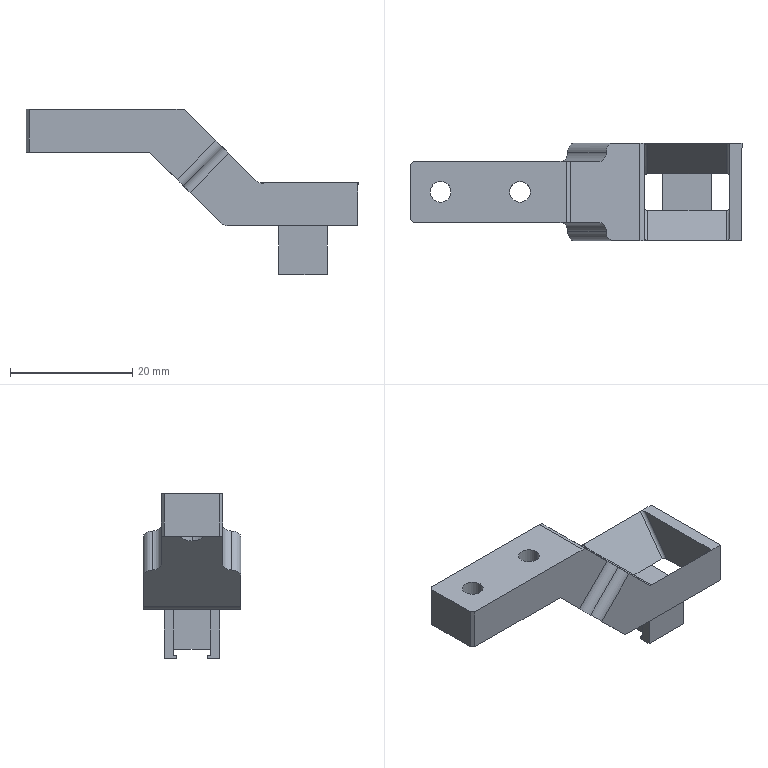Part | 2 solids | 61 faces | box 54.3 x 16 x 27 mm | volume 4932 mm3 | plane 40 | cylinder 21 | commonest cylinder face diameters 3 x8 1 x4 3.4 x4 6 x4 2 x1